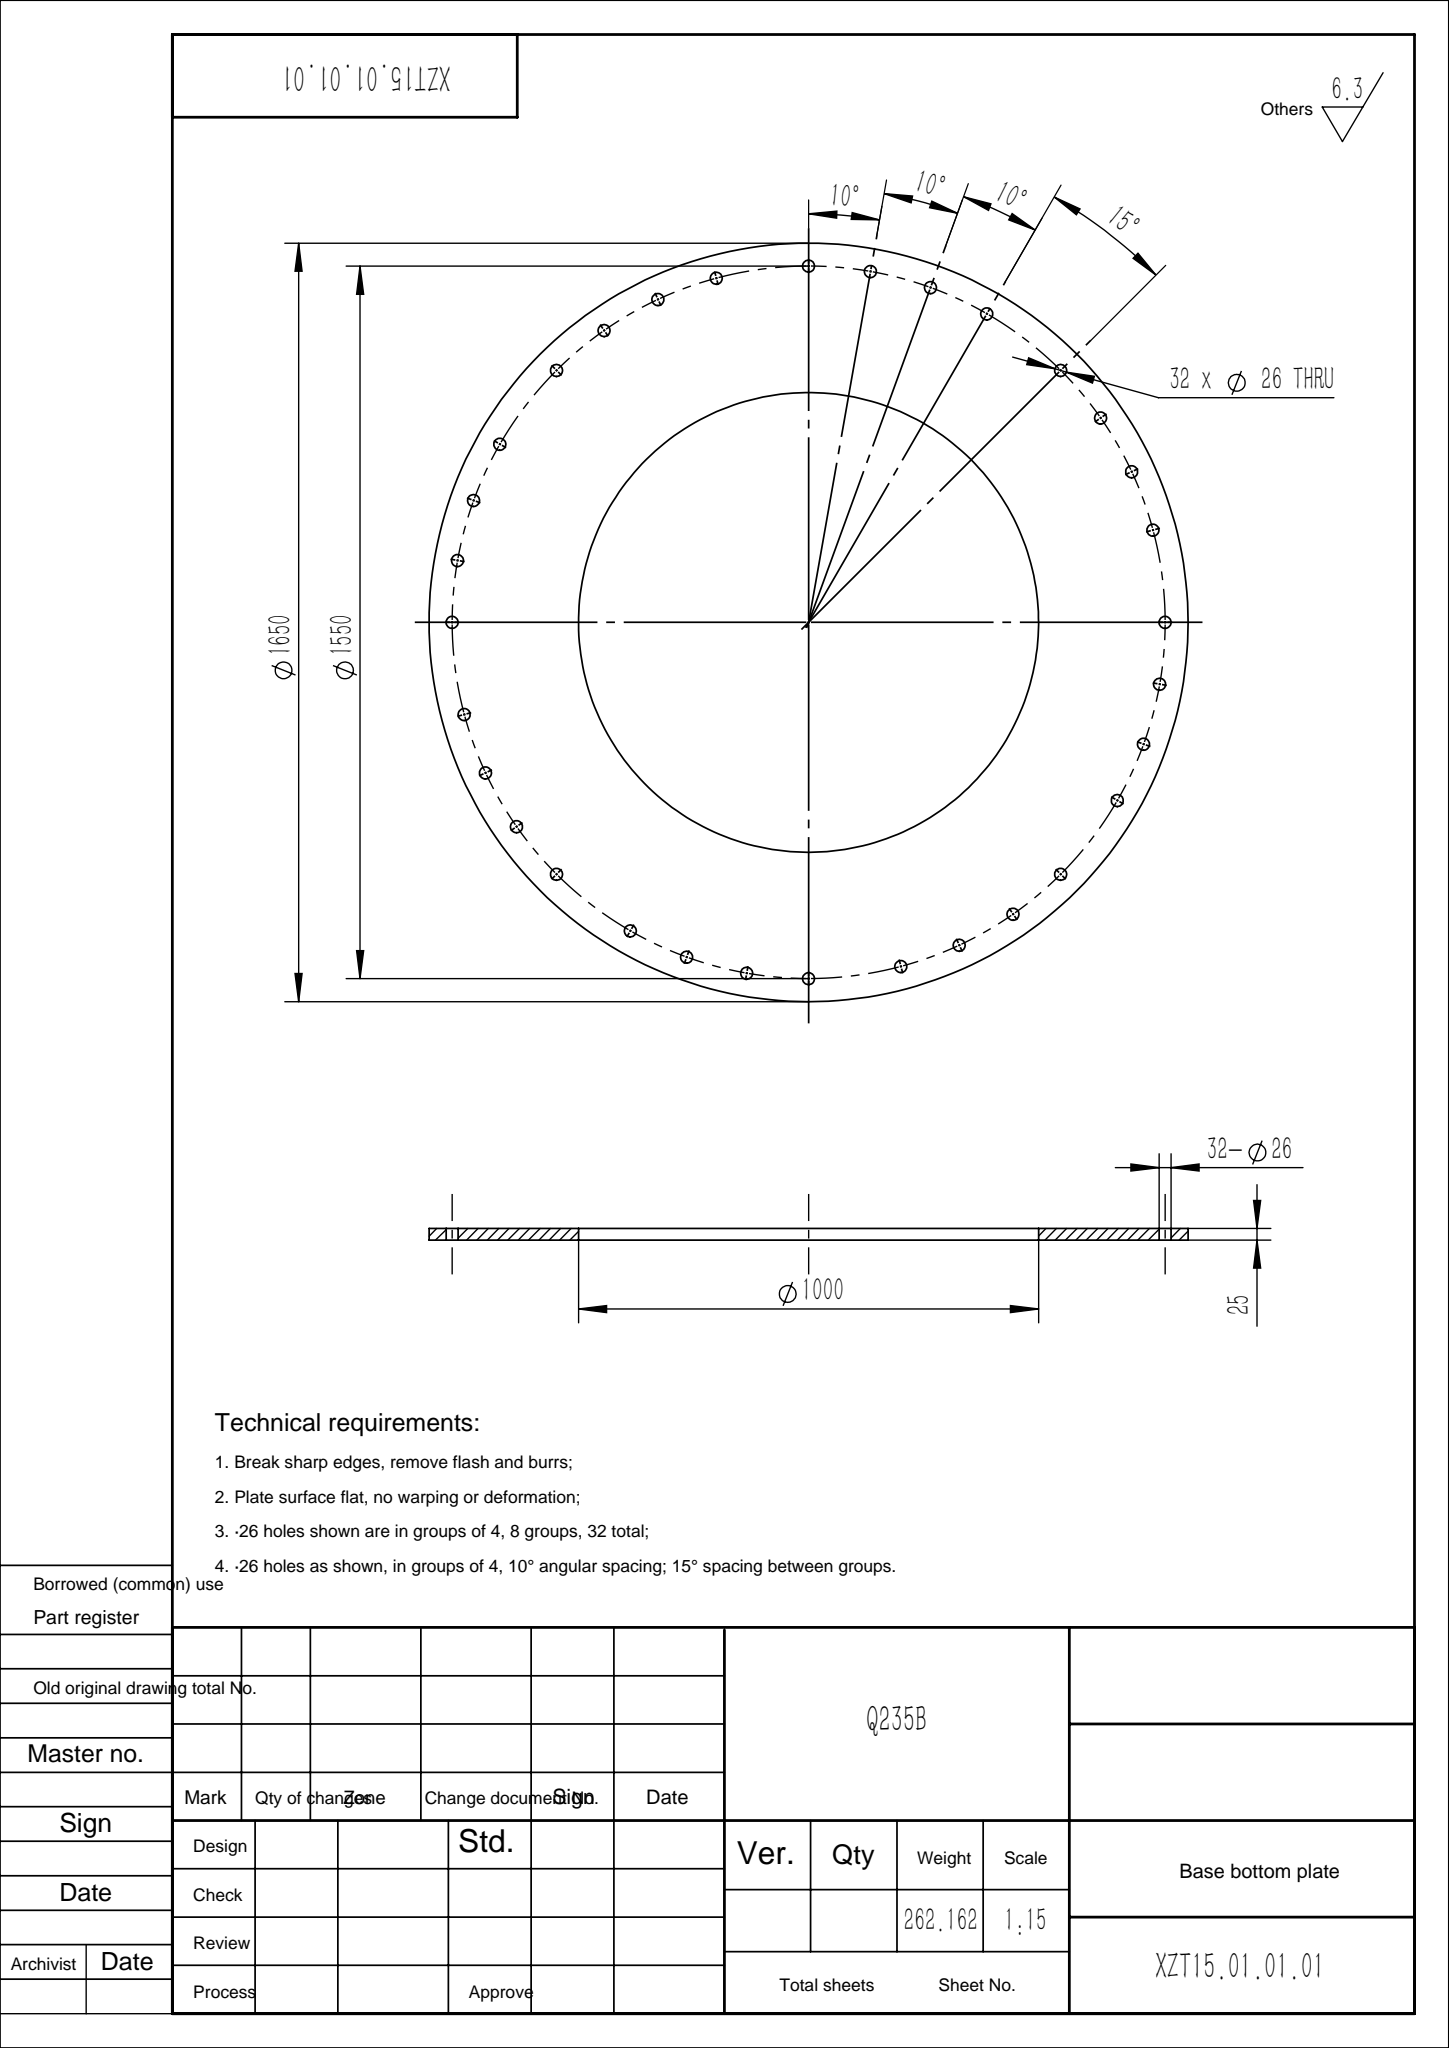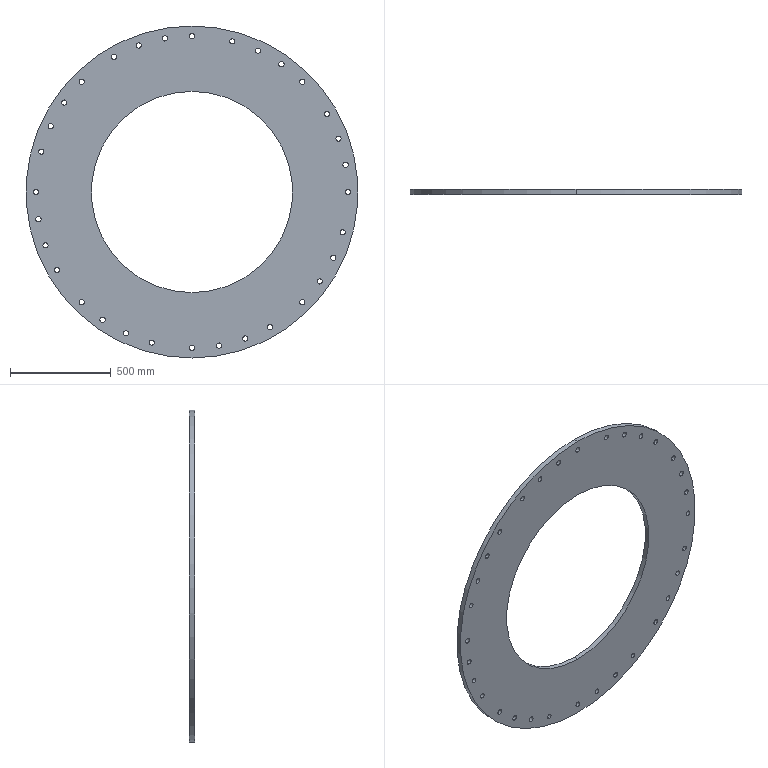Part | SolidWorks | features Extrusion 1, HoleWzd 1 | 1 solid | 70 faces | box 1650 x 25 x 1650 mm | volume 33396465 mm3 | cylinder 68 | plane 2 | commonest cylinder face diameters 26 x64 1000 x2 1650 x2